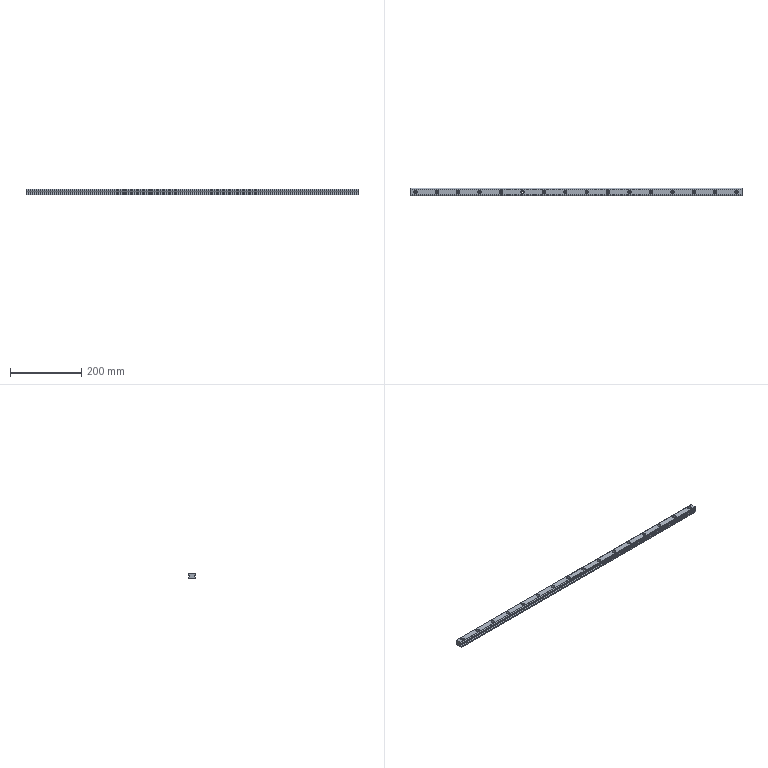Part | SolidWorks | features BaseBody 1 | 1 solid | 104 faces | box 930 x 20 x 16.5 mm | volume 262236 mm3 | cylinder 76 | plane 28 | commonest cylinder face diameters 9.5 x32 6 x20 5.5 x12 0.3 x8 7 x4